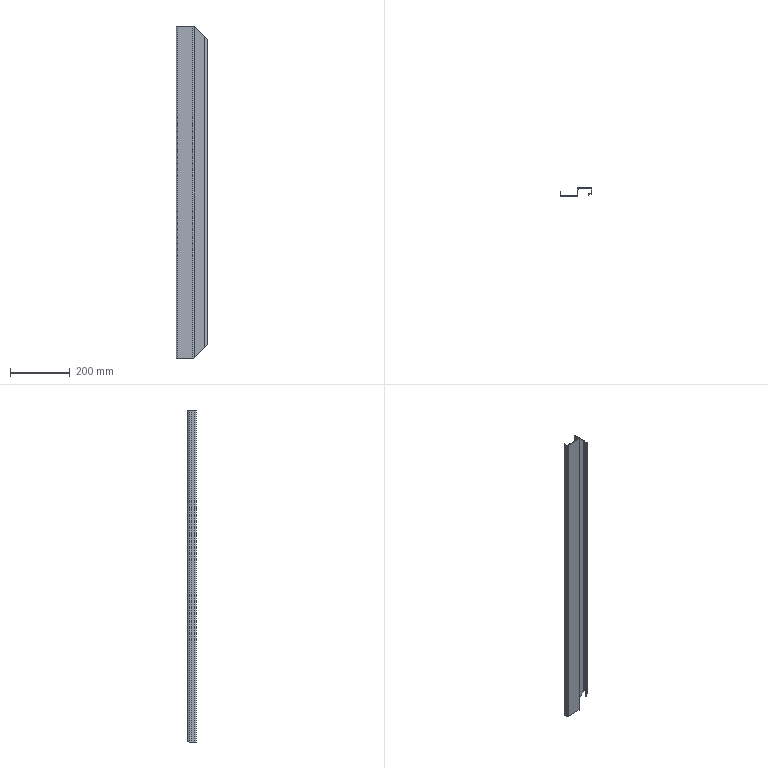Part | STEP file | 750038185 | 1 solid | 38 faces | box 107 x 27 x 1113 mm | volume 364027 mm3 | plane 22 | cylinder 10 | spline 6 | commonest cylinder face diameters 4 x5 8 x5
STEP:
#1=CARTESIAN_POINT('',(-4.,-25.,556.25));
#2=VERTEX_POINT('',#1);
#3=CARTESIAN_POINT('',(-56.,-25.,556.25));
#4=VERTEX_POINT('',#3);
#5=CARTESIAN_POINT('',(0.,-25.,556.25));
#6=DIRECTION('',(-1.,0.,0.));
#7=VECTOR('',#6,1000.);
#8=LINE('',#5,#7);
#9=EDGE_CURVE('',#2,#4,#8,.T.);
#10=ORIENTED_EDGE('',*,*,#9,.T.);
#11=CARTESIAN_POINT('',(-56.,-25.,-556.25));
#12=VERTEX_POINT('',#11);
#13=CARTESIAN_POINT('',(-56.,-25.,556.25));
#14=DIRECTION('',(0.,0.,-1.));
#15=VECTOR('',#14,1000.);
#16=LINE('',#13,#15);
#17=EDGE_CURVE('',#4,#12,#16,.T.);
#18=ORIENTED_EDGE('',*,*,#17,.T.);
#19=CARTESIAN_POINT('',(-4.,-25.,-556.25));
#20=VERTEX_POINT('',#19);
#21=CARTESIAN_POINT('',(0.,-25.,-556.25));
#22=DIRECTION('',(1.,0.,0.));
#23=VECTOR('',#22,1000.);
#24=LINE('',#21,#23);
#25=EDGE_CURVE('',#12,#20,#24,.T.);
#26=ORIENTED_EDGE('',*,*,#25,.T.);
#27=CARTESIAN_POINT('',(-4.,-25.,556.25));
#28=DIRECTION('',(0.,0.,1.));
#29=VECTOR('',#28,1000.);
#30=LINE('',#27,#29);
#31=EDGE_CURVE('',#20,#2,#30,.T.);
#32=ORIENTED_EDGE('',*,*,#31,.T.);
#33=EDGE_LOOP('',(#10,#18,#26,#32));
#34=FACE_OUTER_BOUND('',#33,.T.);
#35=CARTESIAN_POINT('',(0.,-25.,556.25));
#36=DIRECTION('',(0.,-1.,0.));
#37=DIRECTION('',(1.,0.,0.));
#38=AXIS2_PLACEMENT_3D('',#35,#36,#37);
#39=PLANE('',#38);
#40=ADVANCED_FACE('',(#34),#39,.T.);
#41=CARTESIAN_POINT('',(-60.,-21.,556.25));
#42=VERTEX_POINT('',#41);
#43=CARTESIAN_POINT('',(-56.,-21.,556.25));
#44=DIRECTION('',(0.,0.,-1.));
#45=DIRECTION('',(-1.,0.,0.));
#46=AXIS2_PLACEMENT_3D('',#43,#44,#45);
#47=CIRCLE('',#46,4.);
#48=EDGE_CURVE('',#4,#42,#47,.T.);
#49=ORIENTED_EDGE('',*,*,#48,.T.);
#50=CARTESIAN_POINT('',(-60.,-21.,-556.25));
#51=VERTEX_POINT('',#50);
#52=CARTESIAN_POINT('',(-60.,-21.,556.25));
#53=DIRECTION('',(0.,0.,-1.));
#54=VECTOR('',#53,1000.);
#55=LINE('',#52,#54);
#56=EDGE_CURVE('',#42,#51,#55,.T.);
#57=ORIENTED_EDGE('',*,*,#56,.T.);
#58=CARTESIAN_POINT('',(-56.,-21.,-556.25));
#59=DIRECTION('',(0.,0.,1.));
#60=DIRECTION('',(-1.,0.,0.));
#61=AXIS2_PLACEMENT_3D('',#58,#59,#60);
#62=CIRCLE('',#61,4.);
#63=EDGE_CURVE('',#51,#12,#62,.T.);
#64=ORIENTED_EDGE('',*,*,#63,.T.);
#65=ORIENTED_EDGE('',*,*,#17,.F.);
#66=EDGE_LOOP('',(#49,#57,#64,#65));
#67=FACE_OUTER_BOUND('',#66,.T.);
#68=CARTESIAN_POINT('',(-56.,-21.,556.25));
#69=DIRECTION('',(0.,0.,-1.));
#70=DIRECTION('',(-1.,0.,0.));
#71=AXIS2_PLACEMENT_3D('',#68,#69,#70);
#72=CYLINDRICAL_SURFACE('',#71,4.);
#73=ADVANCED_FACE('',(#67),#72,.T.);
#74=CARTESIAN_POINT('',(0.,-21.,556.25));
#75=VERTEX_POINT('',#74);
#76=CARTESIAN_POINT('',(-4.,-21.,556.25));
#77=DIRECTION('',(0.,0.,1.));
#78=DIRECTION('',(-1.,0.,0.));
#79=AXIS2_PLACEMENT_3D('',#76,#77,#78);
#80=CIRCLE('',#79,4.);
#81=EDGE_CURVE('',#2,#75,#80,.T.);
#82=ORIENTED_EDGE('',*,*,#81,.T.);
#83=CARTESIAN_POINT('',(0.,-2.,556.25));
#84=VERTEX_POINT('',#83);
#85=CARTESIAN_POINT('',(0.,-25.,556.25));
#86=DIRECTION('',(0.,1.,0.));
#87=VECTOR('',#86,1000.);
#88=LINE('',#85,#87);
#89=EDGE_CURVE('',#75,#84,#88,.T.);
#90=ORIENTED_EDGE('',*,*,#89,.T.);
#91=CARTESIAN_POINT('',(-2.,-2.,556.25));
#92=VERTEX_POINT('',#91);
#93=CARTESIAN_POINT('',(-60.,-2.,556.25));
#94=DIRECTION('',(-1.,0.,0.));
#95=VECTOR('',#94,1000.);
#96=LINE('',#93,#95);
#97=EDGE_CURVE('',#84,#92,#96,.T.);
#98=ORIENTED_EDGE('',*,*,#97,.T.);
#99=CARTESIAN_POINT('',(-2.,-21.,556.25));
#100=VERTEX_POINT('',#99);
#101=CARTESIAN_POINT('',(-2.,-25.,556.25));
#102=DIRECTION('',(0.,-1.,0.));
#103=VECTOR('',#102,1000.);
#104=LINE('',#101,#103);
#105=EDGE_CURVE('',#92,#100,#104,.T.);
#106=ORIENTED_EDGE('',*,*,#105,.T.);
#107=CARTESIAN_POINT('',(-4.,-23.,556.25));
#108=VERTEX_POINT('',#107);
#109=CARTESIAN_POINT('',(-4.,-21.,556.25));
#110=DIRECTION('',(0.,0.,-1.));
#111=DIRECTION('',(-1.,0.,0.));
#112=AXIS2_PLACEMENT_3D('',#109,#110,#111);
#113=CIRCLE('',#112,2.);
#114=EDGE_CURVE('',#100,#108,#113,.T.);
#115=ORIENTED_EDGE('',*,*,#114,.T.);
#116=CARTESIAN_POINT('',(-56.,-23.,556.25));
#117=VERTEX_POINT('',#116);
#118=CARTESIAN_POINT('',(-60.,-23.,556.25));
#119=DIRECTION('',(-1.,0.,0.));
#120=VECTOR('',#119,1000.);
#121=LINE('',#118,#120);
#122=EDGE_CURVE('',#108,#117,#121,.T.);
#123=ORIENTED_EDGE('',*,*,#122,.T.);
#124=CARTESIAN_POINT('',(-58.,-21.,556.25));
#125=VERTEX_POINT('',#124);
#126=CARTESIAN_POINT('',(-56.,-21.,556.25));
#127=DIRECTION('',(0.,0.,-1.));
#128=DIRECTION('',(-1.,0.,0.));
#129=AXIS2_PLACEMENT_3D('',#126,#127,#128);
#130=CIRCLE('',#129,2.);
#131=EDGE_CURVE('',#117,#125,#130,.T.);
#132=ORIENTED_EDGE('',*,*,#131,.T.);
#133=CARTESIAN_POINT('',(-58.,-10.,556.25));
#134=VERTEX_POINT('',#133);
#135=CARTESIAN_POINT('',(-58.,-25.,556.25));
#136=DIRECTION('',(0.,1.,0.));
#137=VECTOR('',#136,1000.);
#138=LINE('',#135,#137);
#139=EDGE_CURVE('',#125,#134,#138,.T.);
#140=ORIENTED_EDGE('',*,*,#139,.T.);
#141=CARTESIAN_POINT('',(-60.,-10.,556.25));
#142=VERTEX_POINT('',#141);
#143=CARTESIAN_POINT('',(-60.,-10.,556.25));
#144=DIRECTION('',(-1.,0.,0.));
#145=VECTOR('',#144,1000.);
#146=LINE('',#143,#145);
#147=EDGE_CURVE('',#134,#142,#146,.T.);
#148=ORIENTED_EDGE('',*,*,#147,.T.);
#149=CARTESIAN_POINT('',(-60.,-25.,556.25));
#150=DIRECTION('',(0.,-1.,0.));
#151=VECTOR('',#150,1000.);
#152=LINE('',#149,#151);
#153=EDGE_CURVE('',#142,#42,#152,.T.);
#154=ORIENTED_EDGE('',*,*,#153,.T.);
#155=ORIENTED_EDGE('',*,*,#48,.F.);
#156=ORIENTED_EDGE('',*,*,#9,.F.);
#157=EDGE_LOOP('',(#82,#90,#98,#106,#115,#123,#132,#140,#148,#154,#155,#156));
#158=FACE_OUTER_BOUND('',#157,.T.);
#159=CARTESIAN_POINT('',(-60.,-25.,556.25));
#160=DIRECTION('',(0.,0.,1.));
#161=DIRECTION('',(1.,0.,0.));
#162=AXIS2_PLACEMENT_3D('',#159,#160,#161);
#163=PLANE('',#162);
#164=ADVANCED_FACE('',(#158),#163,.T.);
#165=ORIENTED_EDGE('',*,*,#81,.F.);
#166=ORIENTED_EDGE('',*,*,#31,.F.);
#167=CARTESIAN_POINT('',(0.,-21.,-556.25));
#168=VERTEX_POINT('',#167);
#169=CARTESIAN_POINT('',(-4.,-21.,-556.25));
#170=DIRECTION('',(0.,0.,1.));
#171=DIRECTION('',(-1.,0.,0.));
#172=AXIS2_PLACEMENT_3D('',#169,#170,#171);
#173=CIRCLE('',#172,4.);
#174=EDGE_CURVE('',#20,#168,#173,.T.);
#175=ORIENTED_EDGE('',*,*,#174,.T.);
#176=CARTESIAN_POINT('',(0.,-21.,556.25));
#177=DIRECTION('',(0.,0.,1.));
#178=VECTOR('',#177,1000.);
#179=LINE('',#176,#178);
#180=EDGE_CURVE('',#168,#75,#179,.T.);
#181=ORIENTED_EDGE('',*,*,#180,.T.);
#182=EDGE_LOOP('',(#165,#166,#175,#181));
#183=FACE_OUTER_BOUND('',#182,.T.);
#184=CARTESIAN_POINT('',(-4.,-21.,556.25));
#185=DIRECTION('',(0.,0.,-1.));
#186=DIRECTION('',(-1.,0.,0.));
#187=AXIS2_PLACEMENT_3D('',#184,#185,#186);
#188=CYLINDRICAL_SURFACE('',#187,4.);
#189=ADVANCED_FACE('',(#183),#188,.T.);
#190=CARTESIAN_POINT('',(0.,-2.,-556.25));
#191=VERTEX_POINT('',#190);
#192=CARTESIAN_POINT('',(-2.,-2.,-556.25));
#193=VERTEX_POINT('',#192);
#194=CARTESIAN_POINT('',(34.375,-2.,-556.25));
#195=DIRECTION('',(-1.,0.,0.));
#196=VECTOR('',#195,1000.);
#197=LINE('',#194,#196);
#198=EDGE_CURVE('',#191,#193,#197,.T.);
#199=ORIENTED_EDGE('',*,*,#198,.F.);
#200=CARTESIAN_POINT('',(0.,-18.847,-556.25));
#201=DIRECTION('',(0.,1.,0.));
#202=VECTOR('',#201,1000.);
#203=LINE('',#200,#202);
#204=EDGE_CURVE('',#168,#191,#203,.T.);
#205=ORIENTED_EDGE('',*,*,#204,.F.);
#206=ORIENTED_EDGE('',*,*,#174,.F.);
#207=ORIENTED_EDGE('',*,*,#25,.F.);
#208=ORIENTED_EDGE('',*,*,#63,.F.);
#209=CARTESIAN_POINT('',(-60.,-10.,-556.25));
#210=VERTEX_POINT('',#209);
#211=CARTESIAN_POINT('',(-60.,-18.847,-556.25));
#212=DIRECTION('',(0.,-1.,0.));
#213=VECTOR('',#212,1000.);
#214=LINE('',#211,#213);
#215=EDGE_CURVE('',#210,#51,#214,.T.);
#216=ORIENTED_EDGE('',*,*,#215,.F.);
#217=CARTESIAN_POINT('',(-58.,-10.,-556.25));
#218=VERTEX_POINT('',#217);
#219=CARTESIAN_POINT('',(34.375,-10.,-556.25));
#220=DIRECTION('',(-1.,0.,0.));
#221=VECTOR('',#220,1000.);
#222=LINE('',#219,#221);
#223=EDGE_CURVE('',#218,#210,#222,.T.);
#224=ORIENTED_EDGE('',*,*,#223,.F.);
#225=CARTESIAN_POINT('',(-58.,-21.,-556.25));
#226=VERTEX_POINT('',#225);
#227=CARTESIAN_POINT('',(-58.,-18.847,-556.25));
#228=DIRECTION('',(0.,1.,0.));
#229=VECTOR('',#228,1000.);
#230=LINE('',#227,#229);
#231=EDGE_CURVE('',#226,#218,#230,.T.);
#232=ORIENTED_EDGE('',*,*,#231,.F.);
#233=CARTESIAN_POINT('',(-56.,-23.,-556.25));
#234=VERTEX_POINT('',#233);
#235=CARTESIAN_POINT('',(-56.,-21.,-556.25));
#236=DIRECTION('',(0.,0.,-1.));
#237=DIRECTION('',(-1.,0.,0.));
#238=AXIS2_PLACEMENT_3D('',#235,#236,#237);
#239=CIRCLE('',#238,2.);
#240=EDGE_CURVE('',#234,#226,#239,.T.);
#241=ORIENTED_EDGE('',*,*,#240,.F.);
#242=CARTESIAN_POINT('',(-4.,-23.,-556.25));
#243=VERTEX_POINT('',#242);
#244=CARTESIAN_POINT('',(34.375,-23.,-556.25));
#245=DIRECTION('',(-1.,0.,0.));
#246=VECTOR('',#245,1000.);
#247=LINE('',#244,#246);
#248=EDGE_CURVE('',#243,#234,#247,.T.);
#249=ORIENTED_EDGE('',*,*,#248,.F.);
#250=CARTESIAN_POINT('',(-2.,-21.,-556.25));
#251=VERTEX_POINT('',#250);
#252=CARTESIAN_POINT('',(-4.,-21.,-556.25));
#253=DIRECTION('',(0.,0.,-1.));
#254=DIRECTION('',(-1.,0.,0.));
#255=AXIS2_PLACEMENT_3D('',#252,#253,#254);
#256=CIRCLE('',#255,2.);
#257=EDGE_CURVE('',#251,#243,#256,.T.);
#258=ORIENTED_EDGE('',*,*,#257,.F.);
#259=CARTESIAN_POINT('',(-2.,-18.847,-556.25));
#260=DIRECTION('',(0.,-1.,0.));
#261=VECTOR('',#260,1000.);
#262=LINE('',#259,#261);
#263=EDGE_CURVE('',#193,#251,#262,.T.);
#264=ORIENTED_EDGE('',*,*,#263,.F.);
#265=EDGE_LOOP('',(#199,#205,#206,#207,#208,#216,#224,#232,#241,#249,#258,#264));
#266=FACE_OUTER_BOUND('',#265,.T.);
#267=CARTESIAN_POINT('',(34.375,-18.847,-556.25));
#268=DIRECTION('',(0.,0.,1.));
#269=DIRECTION('',(1.,0.,0.));
#270=AXIS2_PLACEMENT_3D('',#267,#268,#269);
#271=PLANE('',#270);
#272=ADVANCED_FACE('',(#266),#271,.F.);
#273=ORIENTED_EDGE('',*,*,#153,.F.);
#274=CARTESIAN_POINT('',(-60.,-10.,556.25));
#275=DIRECTION('',(0.,0.,-1.));
#276=VECTOR('',#275,1000.);
#277=LINE('',#274,#276);
#278=EDGE_CURVE('',#142,#210,#277,.T.);
#279=ORIENTED_EDGE('',*,*,#278,.T.);
#280=ORIENTED_EDGE('',*,*,#215,.T.);
#281=ORIENTED_EDGE('',*,*,#56,.F.);
#282=EDGE_LOOP('',(#273,#279,#280,#281));
#283=FACE_OUTER_BOUND('',#282,.T.);
#284=CARTESIAN_POINT('',(-60.,-25.,556.25));
#285=DIRECTION('',(-1.,0.,0.));
#286=DIRECTION('',(0.,0.,1.));
#287=AXIS2_PLACEMENT_3D('',#284,#285,#286);
#288=PLANE('',#287);
#289=ADVANCED_FACE('',(#283),#288,.T.);
#290=ORIENTED_EDGE('',*,*,#89,.F.);
#291=ORIENTED_EDGE('',*,*,#180,.F.);
#292=ORIENTED_EDGE('',*,*,#204,.T.);
#293=CARTESIAN_POINT('',(0.,-2.,556.25));
#294=DIRECTION('',(0.,0.,1.));
#295=VECTOR('',#294,1000.);
#296=LINE('',#293,#295);
#297=EDGE_CURVE('',#191,#84,#296,.T.);
#298=ORIENTED_EDGE('',*,*,#297,.T.);
#299=EDGE_LOOP('',(#290,#291,#292,#298));
#300=FACE_OUTER_BOUND('',#299,.T.);
#301=CARTESIAN_POINT('',(0.,0.,556.25));
#302=DIRECTION('',(1.,0.,0.));
#303=DIRECTION('',(0.,1.,0.));
#304=AXIS2_PLACEMENT_3D('',#301,#302,#303);
#305=PLANE('',#304);
#306=ADVANCED_FACE('',(#300),#305,.T.);
#307=ORIENTED_EDGE('',*,*,#223,.T.);
#308=ORIENTED_EDGE('',*,*,#278,.F.);
#309=ORIENTED_EDGE('',*,*,#147,.F.);
#310=CARTESIAN_POINT('',(-58.,-10.,556.25));
#311=DIRECTION('',(0.,0.,-1.));
#312=VECTOR('',#311,1000.);
#313=LINE('',#310,#312);
#314=EDGE_CURVE('',#134,#218,#313,.T.);
#315=ORIENTED_EDGE('',*,*,#314,.T.);
#316=EDGE_LOOP('',(#307,#308,#309,#315));
#317=FACE_OUTER_BOUND('',#316,.T.);
#318=CARTESIAN_POINT('',(-60.,-10.,556.25));
#319=DIRECTION('',(0.,1.,0.));
#320=DIRECTION('',(0.,0.,1.));
#321=AXIS2_PLACEMENT_3D('',#318,#319,#320);
#322=PLANE('',#321);
#323=ADVANCED_FACE('',(#317),#322,.T.);
#324=ORIENTED_EDGE('',*,*,#314,.F.);
#325=ORIENTED_EDGE('',*,*,#139,.F.);
#326=CARTESIAN_POINT('',(-58.,-21.,556.25));
#327=DIRECTION('',(0.,0.,1.));
#328=VECTOR('',#327,1000.);
#329=LINE('',#326,#328);
#330=EDGE_CURVE('',#226,#125,#329,.T.);
#331=ORIENTED_EDGE('',*,*,#330,.F.);
#332=ORIENTED_EDGE('',*,*,#231,.T.);
#333=EDGE_LOOP('',(#324,#325,#331,#332));
#334=FACE_OUTER_BOUND('',#333,.T.);
#335=CARTESIAN_POINT('',(-58.,-25.,556.25));
#336=DIRECTION('',(-1.,0.,0.));
#337=DIRECTION('',(0.,0.,1.));
#338=AXIS2_PLACEMENT_3D('',#335,#336,#337);
#339=PLANE('',#338);
#340=ADVANCED_FACE('',(#334),#339,.F.);
#341=ORIENTED_EDGE('',*,*,#330,.T.);
#342=ORIENTED_EDGE('',*,*,#131,.F.);
#343=CARTESIAN_POINT('',(-56.,-23.,556.25));
#344=DIRECTION('',(0.,0.,1.));
#345=VECTOR('',#344,1000.);
#346=LINE('',#343,#345);
#347=EDGE_CURVE('',#234,#117,#346,.T.);
#348=ORIENTED_EDGE('',*,*,#347,.F.);
#349=ORIENTED_EDGE('',*,*,#240,.T.);
#350=EDGE_LOOP('',(#341,#342,#348,#349));
#351=FACE_OUTER_BOUND('',#350,.T.);
#352=CARTESIAN_POINT('',(-56.,-21.,556.25));
#353=DIRECTION('',(0.,0.,-1.));
#354=DIRECTION('',(-1.,0.,0.));
#355=AXIS2_PLACEMENT_3D('',#352,#353,#354);
#356=CYLINDRICAL_SURFACE('',#355,2.);
#357=ADVANCED_FACE('',(#351),#356,.F.);
#358=ORIENTED_EDGE('',*,*,#347,.T.);
#359=ORIENTED_EDGE('',*,*,#122,.F.);
#360=CARTESIAN_POINT('',(-4.,-23.,556.25));
#361=DIRECTION('',(0.,0.,1.));
#362=VECTOR('',#361,1000.);
#363=LINE('',#360,#362);
#364=EDGE_CURVE('',#243,#108,#363,.T.);
#365=ORIENTED_EDGE('',*,*,#364,.F.);
#366=ORIENTED_EDGE('',*,*,#248,.T.);
#367=EDGE_LOOP('',(#358,#359,#365,#366));
#368=FACE_OUTER_BOUND('',#367,.T.);
#369=CARTESIAN_POINT('',(0.,-23.,556.25));
#370=DIRECTION('',(0.,-1.,0.));
#371=DIRECTION('',(1.,0.,0.));
#372=AXIS2_PLACEMENT_3D('',#369,#370,#371);
#373=PLANE('',#372);
#374=ADVANCED_FACE('',(#368),#373,.F.);
#375=ORIENTED_EDGE('',*,*,#364,.T.);
#376=ORIENTED_EDGE('',*,*,#114,.F.);
#377=CARTESIAN_POINT('',(-2.,-21.,556.25));
#378=DIRECTION('',(0.,0.,1.));
#379=VECTOR('',#378,1000.);
#380=LINE('',#377,#379);
#381=EDGE_CURVE('',#251,#100,#380,.T.);
#382=ORIENTED_EDGE('',*,*,#381,.F.);
#383=ORIENTED_EDGE('',*,*,#257,.T.);
#384=EDGE_LOOP('',(#375,#376,#382,#383));
#385=FACE_OUTER_BOUND('',#384,.T.);
#386=CARTESIAN_POINT('',(-4.,-21.,556.25));
#387=DIRECTION('',(0.,0.,-1.));
#388=DIRECTION('',(-1.,0.,0.));
#389=AXIS2_PLACEMENT_3D('',#386,#387,#388);
#390=CYLINDRICAL_SURFACE('',#389,2.);
#391=ADVANCED_FACE('',(#385),#390,.F.);
#392=ORIENTED_EDGE('',*,*,#381,.T.);
#393=ORIENTED_EDGE('',*,*,#105,.F.);
#394=CARTESIAN_POINT('',(-2.,-2.,556.25));
#395=DIRECTION('',(0.,0.,1.));
#396=VECTOR('',#395,1000.);
#397=LINE('',#394,#396);
#398=EDGE_CURVE('',#193,#92,#397,.T.);
#399=ORIENTED_EDGE('',*,*,#398,.F.);
#400=ORIENTED_EDGE('',*,*,#263,.T.);
#401=EDGE_LOOP('',(#392,#393,#399,#400));
#402=FACE_OUTER_BOUND('',#401,.T.);
#403=CARTESIAN_POINT('',(-2.,0.,556.25));
#404=DIRECTION('',(1.,0.,0.));
#405=DIRECTION('',(0.,1.,0.));
#406=AXIS2_PLACEMENT_3D('',#403,#404,#405);
#407=PLANE('',#406);
#408=ADVANCED_FACE('',(#402),#407,.F.);
#409=CARTESIAN_POINT('',(2.,0.,554.25));
#410=VERTEX_POINT('',#409);
#411=CARTESIAN_POINT('',(2.,2.,554.25));
#412=VERTEX_POINT('',#411);
#413=CARTESIAN_POINT('',(2.,1.,554.25));
#414=DIRECTION('',(0.,1.,0.));
#415=VECTOR('',#414,1000.);
#416=LINE('',#413,#415);
#417=EDGE_CURVE('',#410,#412,#416,.T.);
#418=ORIENTED_EDGE('',*,*,#417,.T.);
#419=CARTESIAN_POINT('',(2.,2.,554.25));
#420=CARTESIAN_POINT('',(-0.6667,2.,555.583));
#421=CARTESIAN_POINT('',(-2.,0.,556.25));
#422=CARTESIAN_POINT('',(-2.,-2.,556.25));
#423=(BOUNDED_CURVE()B_SPLINE_CURVE(3,(#419,#420,#421,#422),.UNSPECIFIED.,.F.,.F.)B_SPLINE_CURVE_WITH_KNOTS((4,4),(0.,0.006622),.UNSPECIFIED.)CURVE()GEOMETRIC_REPRESENTATION_ITEM()RATIONAL_B_SPLINE_CURVE((0.5,0.5,0.6667,1.))REPRESENTATION_ITEM(''));
#424=EDGE_CURVE('',#412,#92,#423,.T.);
#425=ORIENTED_EDGE('',*,*,#424,.T.);
#426=ORIENTED_EDGE('',*,*,#97,.F.);
#427=CARTESIAN_POINT('',(0.,-2.,556.25));
#428=CARTESIAN_POINT('',(0.,-1.,556.25));
#429=CARTESIAN_POINT('',(0.6667,0.,555.583));
#430=CARTESIAN_POINT('',(2.,0.,554.25));
#431=(BOUNDED_CURVE()B_SPLINE_CURVE(3,(#427,#428,#429,#430),.UNSPECIFIED.,.F.,.F.)B_SPLINE_CURVE_WITH_KNOTS((4,4),(0.,0.003854),.UNSPECIFIED.)CURVE()GEOMETRIC_REPRESENTATION_ITEM()RATIONAL_B_SPLINE_CURVE((1.,0.6667,0.5,0.5))REPRESENTATION_ITEM(''));
#432=EDGE_CURVE('',#84,#410,#431,.T.);
#433=ORIENTED_EDGE('',*,*,#432,.T.);
#434=EDGE_LOOP('',(#418,#425,#426,#433));
#435=FACE_OUTER_BOUND('',#434,.T.);
#436=CARTESIAN_POINT('',(4.,-2.,552.25));
#437=CARTESIAN_POINT('',(4.667,-2.,552.25));
#438=CARTESIAN_POINT('',(5.333,-2.,552.25));
#439=CARTESIAN_POINT('',(6.,-2.,552.25));
#440=CARTESIAN_POINT('',(4.,-6.,552.25));
#441=CARTESIAN_POINT('',(4.667,-7.333,552.25));
#442=CARTESIAN_POINT('',(5.333,-8.667,552.25));
#443=CARTESIAN_POINT('',(6.,-10.,552.25));
#444=CARTESIAN_POINT('',(0.,-6.,556.25));
#445=CARTESIAN_POINT('',(-0.6667,-7.333,556.25));
#446=CARTESIAN_POINT('',(-1.333,-8.667,556.25));
#447=CARTESIAN_POINT('',(-2.,-10.,556.25));
#448=CARTESIAN_POINT('',(0.,-2.,556.25));
#449=CARTESIAN_POINT('',(-0.6667,-2.,556.25));
#450=CARTESIAN_POINT('',(-1.333,-2.,556.25));
#451=CARTESIAN_POINT('',(-2.,-2.,556.25));
#452=CARTESIAN_POINT('',(0.,2.,556.25));
#453=CARTESIAN_POINT('',(-0.6667,3.333,556.25));
#454=CARTESIAN_POINT('',(-1.333,4.667,556.25));
#455=CARTESIAN_POINT('',(-2.,6.,556.25));
#456=CARTESIAN_POINT('',(4.,2.,552.25));
#457=CARTESIAN_POINT('',(4.667,3.333,552.25));
#458=CARTESIAN_POINT('',(5.333,4.667,552.25));
#459=CARTESIAN_POINT('',(6.,6.,552.25));
#460=CARTESIAN_POINT('',(4.,-2.,552.25));
#461=CARTESIAN_POINT('',(4.667,-2.,552.25));
#462=CARTESIAN_POINT('',(5.333,-2.,552.25));
#463=CARTESIAN_POINT('',(6.,-2.,552.25));
#464=(BOUNDED_SURFACE()B_SPLINE_SURFACE(3,3,((#436,#437,#438,#439),(#440,#441,#442,#443),(#444,#445,#446,#447),(#448,#449,#450,#451),(#452,#453,#454,#455),(#456,#457,#458,#459),(#460,#461,#462,#463)),.UNSPECIFIED.,.T.,.F.,.F.)B_SPLINE_SURFACE_WITH_KNOTS((4,3,4),(4,4),(0.,0.5,1.),(0.,1.),.UNSPECIFIED.)GEOMETRIC_REPRESENTATION_ITEM()RATIONAL_B_SPLINE_SURFACE(((1.,1.,1.,1.),(0.3333,0.3333,0.3333,0.3333),(0.3333,0.3333,0.3333,0.3333),(1.,1.,1.,1.),(0.3333,0.3333,0.3333,0.3333),(0.3333,0.3333,0.3333,0.3333),(1.,1.,1.,1.)))REPRESENTATION_ITEM('')SURFACE());
#465=ADVANCED_FACE('',(#435),#464,.T.);
#466=ORIENTED_EDGE('',*,*,#198,.T.);
#467=CARTESIAN_POINT('',(2.,2.,-554.25));
#468=VERTEX_POINT('',#467);
#469=CARTESIAN_POINT('',(-2.,-2.,-556.25));
#470=CARTESIAN_POINT('',(-2.,0.,-556.25));
#471=CARTESIAN_POINT('',(-0.6667,2.,-555.583));
#472=CARTESIAN_POINT('',(2.,2.,-554.25));
#473=(BOUNDED_CURVE()B_SPLINE_CURVE(3,(#469,#470,#471,#472),.UNSPECIFIED.,.F.,.F.)B_SPLINE_CURVE_WITH_KNOTS((4,4),(0.,0.006696),.UNSPECIFIED.)CURVE()GEOMETRIC_REPRESENTATION_ITEM()RATIONAL_B_SPLINE_CURVE((1.,0.6667,0.5,0.5))REPRESENTATION_ITEM(''));
#474=EDGE_CURVE('',#193,#468,#473,.T.);
#475=ORIENTED_EDGE('',*,*,#474,.T.);
#476=CARTESIAN_POINT('',(2.,0.,-554.25));
#477=VERTEX_POINT('',#476);
#478=CARTESIAN_POINT('',(2.,1.,-554.25));
#479=DIRECTION('',(0.,-1.,0.));
#480=VECTOR('',#479,1000.);
#481=LINE('',#478,#480);
#482=EDGE_CURVE('',#468,#477,#481,.T.);
#483=ORIENTED_EDGE('',*,*,#482,.T.);
#484=CARTESIAN_POINT('',(2.,0.,-554.25));
#485=CARTESIAN_POINT('',(0.6667,0.,-555.583));
#486=CARTESIAN_POINT('',(0.,-1.,-556.25));
#487=CARTESIAN_POINT('',(0.,-2.,-556.25));
#488=(BOUNDED_CURVE()B_SPLINE_CURVE(3,(#484,#485,#486,#487),.UNSPECIFIED.,.F.,.T.)B_SPLINE_CURVE_WITH_KNOTS((4,4),(0.,0.003785),.UNSPECIFIED.)CURVE()GEOMETRIC_REPRESENTATION_ITEM()RATIONAL_B_SPLINE_CURVE((0.5,0.5,0.6667,1.))REPRESENTATION_ITEM(''));
#489=EDGE_CURVE('',#477,#191,#488,.T.);
#490=ORIENTED_EDGE('',*,*,#489,.T.);
#491=EDGE_LOOP('',(#466,#475,#483,#490));
#492=FACE_OUTER_BOUND('',#491,.T.);
#493=CARTESIAN_POINT('',(0.,-2.,-556.25));
#494=CARTESIAN_POINT('',(-0.6667,-2.,-556.25));
#495=CARTESIAN_POINT('',(-1.333,-2.,-556.25));
#496=CARTESIAN_POINT('',(-2.,-2.,-556.25));
#497=CARTESIAN_POINT('',(0.,-6.,-556.25));
#498=CARTESIAN_POINT('',(-0.6667,-7.333,-556.25));
#499=CARTESIAN_POINT('',(-1.333,-8.667,-556.25));
#500=CARTESIAN_POINT('',(-2.,-10.,-556.25));
#501=CARTESIAN_POINT('',(4.,-6.,-552.25));
#502=CARTESIAN_POINT('',(4.667,-7.333,-552.25));
#503=CARTESIAN_POINT('',(5.333,-8.667,-552.25));
#504=CARTESIAN_POINT('',(6.,-10.,-552.25));
#505=CARTESIAN_POINT('',(4.,-2.,-552.25));
#506=CARTESIAN_POINT('',(4.667,-2.,-552.25));
#507=CARTESIAN_POINT('',(5.333,-2.,-552.25));
#508=CARTESIAN_POINT('',(6.,-2.,-552.25));
#509=CARTESIAN_POINT('',(4.,2.,-552.25));
#510=CARTESIAN_POINT('',(4.667,3.333,-552.25));
#511=CARTESIAN_POINT('',(5.333,4.667,-552.25));
#512=CARTESIAN_POINT('',(6.,6.,-552.25));
#513=CARTESIAN_POINT('',(0.,2.,-556.25));
#514=CARTESIAN_POINT('',(-0.6667,3.333,-556.25));
#515=CARTESIAN_POINT('',(-1.333,4.667,-556.25));
#516=CARTESIAN_POINT('',(-2.,6.,-556.25));
#517=CARTESIAN_POINT('',(0.,-2.,-556.25));
#518=CARTESIAN_POINT('',(-0.6667,-2.,-556.25));
#519=CARTESIAN_POINT('',(-1.333,-2.,-556.25));
#520=CARTESIAN_POINT('',(-2.,-2.,-556.25));
#521=(BOUNDED_SURFACE()B_SPLINE_SURFACE(3,3,((#493,#494,#495,#496),(#497,#498,#499,#500),(#501,#502,#503,#504),(#505,#506,#507,#508),(#509,#510,#511,#512),(#513,#514,#515,#516),(#517,#518,#519,#520)),.UNSPECIFIED.,.T.,.F.,.F.)B_SPLINE_SURFACE_WITH_KNOTS((4,3,4),(4,4),(0.,0.5,1.),(0.,1.),.UNSPECIFIED.)GEOMETRIC_REPRESENTATION_ITEM()RATIONAL_B_SPLINE_SURFACE(((1.,1.,1.,1.),(0.3333,0.3333,0.3333,0.3333),(0.3333,0.3333,0.3333,0.3333),(1.,1.,1.,1.),(0.3333,0.3333,0.3333,0.3333),(0.3333,0.3333,0.3333,0.3333),(1.,1.,1.,1.)))REPRESENTATION_ITEM('')SURFACE());
#522=ADVANCED_FACE('',(#492),#521,.T.);
#523=ORIENTED_EDGE('',*,*,#297,.F.);
#524=ORIENTED_EDGE('',*,*,#489,.F.);
#525=CARTESIAN_POINT('',(2.,0.,556.25));
#526=DIRECTION('',(0.,0.,-1.));
#527=VECTOR('',#526,1000.);
#528=LINE('',#525,#527);
#529=EDGE_CURVE('',#410,#477,#528,.T.);
#530=ORIENTED_EDGE('',*,*,#529,.F.);
#531=ORIENTED_EDGE('',*,*,#432,.F.);
#532=EDGE_LOOP('',(#523,#524,#530,#531));
#533=FACE_OUTER_BOUND('',#532,.T.);
#534=CARTESIAN_POINT('',(2.,-2.,556.25));
#535=DIRECTION('',(0.,0.,-1.));
#536=DIRECTION('',(-1.,0.,0.));
#537=AXIS2_PLACEMENT_3D('',#534,#535,#536);
#538=CYLINDRICAL_SURFACE('',#537,2.);
#539=ADVANCED_FACE('',(#533),#538,.F.);
#540=CARTESIAN_POINT('',(2.,2.,556.25));
#541=DIRECTION('',(0.,0.,-1.));
#542=VECTOR('',#541,1000.);
#543=LINE('',#540,#542);
#544=EDGE_CURVE('',#412,#468,#543,.T.);
#545=ORIENTED_EDGE('',*,*,#544,.T.);
#546=ORIENTED_EDGE('',*,*,#474,.F.);
#547=ORIENTED_EDGE('',*,*,#398,.T.);
#548=ORIENTED_EDGE('',*,*,#424,.F.);
#549=EDGE_LOOP('',(#545,#546,#547,#548));
#550=FACE_OUTER_BOUND('',#549,.T.);
#551=CARTESIAN_POINT('',(2.,-2.,556.25));
#552=DIRECTION('',(0.,0.,-1.));
#553=DIRECTION('',(-1.,0.,0.));
#554=AXIS2_PLACEMENT_3D('',#551,#552,#553);
#555=CYLINDRICAL_SURFACE('',#554,4.);
#556=ADVANCED_FACE('',(#550),#555,.T.);
#557=CARTESIAN_POINT('',(43.,0.,513.25));
#558=VERTEX_POINT('',#557);
#559=CARTESIAN_POINT('',(22.5,0.,533.75));
#560=DIRECTION('',(-0.7071,0.,0.7071));
#561=VECTOR('',#560,1000.);
#562=LINE('',#559,#561);
#563=EDGE_CURVE('',#558,#410,#562,.T.);
#564=ORIENTED_EDGE('',*,*,#563,.F.);
#565=CARTESIAN_POINT('',(43.,2.,513.25));
#566=VERTEX_POINT('',#565);
#567=CARTESIAN_POINT('',(43.,0.,513.25));
#568=DIRECTION('',(0.,-1.,0.));
#569=VECTOR('',#568,1000.);
#570=LINE('',#567,#569);
#571=EDGE_CURVE('',#566,#558,#570,.T.);
#572=ORIENTED_EDGE('',*,*,#571,.F.);
#573=CARTESIAN_POINT('',(22.5,2.,533.75));
#574=DIRECTION('',(0.7071,0.,-0.7071));
#575=VECTOR('',#574,1000.);
#576=LINE('',#573,#575);
#577=EDGE_CURVE('',#412,#566,#576,.T.);
#578=ORIENTED_EDGE('',*,*,#577,.F.);
#579=ORIENTED_EDGE('',*,*,#417,.F.);
#580=EDGE_LOOP('',(#564,#572,#578,#579));
#581=FACE_OUTER_BOUND('',#580,.T.);
#582=CARTESIAN_POINT('',(22.5,0.,533.75));
#583=DIRECTION('',(-0.7071,0.,-0.7071));
#584=DIRECTION('',(-0.7071,0.,0.7071));
#585=AXIS2_PLACEMENT_3D('',#582,#583,#584);
#586=PLANE('',#585);
#587=ADVANCED_FACE('',(#581),#586,.F.);
#588=CARTESIAN_POINT('',(43.,0.,-513.25));
#589=VERTEX_POINT('',#588);
#590=CARTESIAN_POINT('',(578.75,0.,22.5));
#591=DIRECTION('',(0.7071,0.,0.7071));
#592=VECTOR('',#591,1000.);
#593=LINE('',#590,#592);
#594=EDGE_CURVE('',#477,#589,#593,.T.);
#595=ORIENTED_EDGE('',*,*,#594,.F.);
#596=ORIENTED_EDGE('',*,*,#482,.F.);
#597=CARTESIAN_POINT('',(43.,2.,-513.25));
#598=VERTEX_POINT('',#597);
#599=CARTESIAN_POINT('',(578.75,2.,22.5));
#600=DIRECTION('',(-0.7071,0.,-0.7071));
#601=VECTOR('',#600,1000.);
#602=LINE('',#599,#601);
#603=EDGE_CURVE('',#598,#468,#602,.T.);
#604=ORIENTED_EDGE('',*,*,#603,.F.);
#605=CARTESIAN_POINT('',(43.,0.,-513.25));
#606=DIRECTION('',(0.,1.,0.));
#607=VECTOR('',#606,1000.);
#608=LINE('',#605,#607);
#609=EDGE_CURVE('',#589,#598,#608,.T.);
#610=ORIENTED_EDGE('',*,*,#609,.F.);
#611=EDGE_LOOP('',(#595,#596,#604,#610));
#612=FACE_OUTER_BOUND('',#611,.T.);
#613=CARTESIAN_POINT('',(578.75,0.,22.5));
#614=DIRECTION('',(-0.7071,0.,0.7071));
#615=DIRECTION('',(0.7071,0.,0.7071));
#616=AXIS2_PLACEMENT_3D('',#613,#614,#615);
#617=PLANE('',#616);
#618=ADVANCED_FACE('',(#612),#617,.F.);
#619=ORIENTED_EDGE('',*,*,#594,.T.);
#620=CARTESIAN_POINT('',(43.,0.,556.25));
#621=DIRECTION('',(0.,0.,1.));
#622=VECTOR('',#621,1000.);
#623=LINE('',#620,#622);
#624=EDGE_CURVE('',#589,#558,#623,.T.);
#625=ORIENTED_EDGE('',*,*,#624,.T.);
#626=ORIENTED_EDGE('',*,*,#563,.T.);
#627=ORIENTED_EDGE('',*,*,#529,.T.);
#628=EDGE_LOOP('',(#619,#625,#626,#627));
#629=FACE_OUTER_BOUND('',#628,.T.);
#630=CARTESIAN_POINT('',(45.,0.,556.25));
#631=DIRECTION('',(0.,-1.,0.));
#632=DIRECTION('',(0.,0.,-1.));
#633=AXIS2_PLACEMENT_3D('',#630,#631,#632);
#634=PLANE('',#633);
#635=ADVANCED_FACE('',(#629),#634,.T.);
#636=ORIENTED_EDGE('',*,*,#577,.T.);
#637=CARTESIAN_POINT('',(43.,2.,556.25));
#638=DIRECTION('',(0.,0.,1.));
#639=VECTOR('',#638,1000.);
#640=LINE('',#637,#639);
#641=EDGE_CURVE('',#598,#566,#640,.T.);
#642=ORIENTED_EDGE('',*,*,#641,.F.);
#643=ORIENTED_EDGE('',*,*,#603,.T.);
#644=ORIENTED_EDGE('',*,*,#544,.F.);
#645=EDGE_LOOP('',(#636,#642,#643,#644));
#646=FACE_OUTER_BOUND('',#645,.T.);
#647=CARTESIAN_POINT('',(45.,2.,556.25));
#648=DIRECTION('',(0.,-1.,0.));
#649=DIRECTION('',(0.,0.,-1.));
#650=AXIS2_PLACEMENT_3D('',#647,#648,#649);
#651=PLANE('',#650);
#652=ADVANCED_FACE('',(#646),#651,.F.);
#653=CARTESIAN_POINT('',(47.,-2.,509.25));
#654=VERTEX_POINT('',#653);
#655=CARTESIAN_POINT('',(47.,-2.,509.25));
#656=CARTESIAN_POINT('',(47.,0.,509.25));
#657=CARTESIAN_POINT('',(45.667,2.,510.583));
#658=CARTESIAN_POINT('',(43.,2.,513.25));
#659=(BOUNDED_CURVE()B_SPLINE_CURVE(3,(#655,#656,#657,#658),.UNSPECIFIED.,.F.,.F.)B_SPLINE_CURVE_WITH_KNOTS((4,4),(0.,0.007712),.UNSPECIFIED.)CURVE()GEOMETRIC_REPRESENTATION_ITEM()RATIONAL_B_SPLINE_CURVE((1.,0.6667,0.5,0.5))REPRESENTATION_ITEM(''));
#660=EDGE_CURVE('',#654,#566,#659,.T.);
#661=ORIENTED_EDGE('',*,*,#660,.T.);
#662=ORIENTED_EDGE('',*,*,#571,.T.);
#663=CARTESIAN_POINT('',(45.,-2.,509.25));
#664=VERTEX_POINT('',#663);
#665=CARTESIAN_POINT('',(43.,0.,513.25));
#666=CARTESIAN_POINT('',(44.333,0.,510.583));
#667=CARTESIAN_POINT('',(45.,-1.,509.25));
#668=CARTESIAN_POINT('',(45.,-2.,509.25));
#669=(BOUNDED_CURVE()B_SPLINE_CURVE(3,(#665,#666,#667,#668),.UNSPECIFIED.,.F.,.F.)B_SPLINE_CURVE_WITH_KNOTS((4,4),(0.,0.005228),.UNSPECIFIED.)CURVE()GEOMETRIC_REPRESENTATION_ITEM()RATIONAL_B_SPLINE_CURVE((0.5,0.5,0.6667,1.))REPRESENTATION_ITEM(''));
#670=EDGE_CURVE('',#558,#664,#669,.T.);
#671=ORIENTED_EDGE('',*,*,#670,.T.);
#672=CARTESIAN_POINT('',(46.,-2.,509.25));
#673=DIRECTION('',(1.,0.,0.));
#674=VECTOR('',#673,1000.);
#675=LINE('',#672,#674);
#676=EDGE_CURVE('',#664,#654,#675,.T.);
#677=ORIENTED_EDGE('',*,*,#676,.T.);
#678=EDGE_LOOP('',(#661,#662,#671,#677));
#679=FACE_OUTER_BOUND('',#678,.T.);
#680=CARTESIAN_POINT('',(45.,-2.,509.25));
#681=CARTESIAN_POINT('',(45.667,-2.,509.25));
#682=CARTESIAN_POINT('',(46.333,-2.,509.25));
#683=CARTESIAN_POINT('',(47.,-2.,509.25));
#684=CARTESIAN_POINT('',(45.,-6.,509.25));
#685=CARTESIAN_POINT('',(45.667,-7.333,509.25));
#686=CARTESIAN_POINT('',(46.333,-8.667,509.25));
#687=CARTESIAN_POINT('',(47.,-10.,509.25));
#688=CARTESIAN_POINT('',(41.,-6.,517.25));
#689=CARTESIAN_POINT('',(40.333,-7.333,517.25));
#690=CARTESIAN_POINT('',(39.667,-8.667,517.25));
#691=CARTESIAN_POINT('',(39.,-10.,517.25));
#692=CARTESIAN_POINT('',(41.,-2.,517.25));
#693=CARTESIAN_POINT('',(40.333,-2.,517.25));
#694=CARTESIAN_POINT('',(39.667,-2.,517.25));
#695=CARTESIAN_POINT('',(39.,-2.,517.25));
#696=CARTESIAN_POINT('',(41.,2.,517.25));
#697=CARTESIAN_POINT('',(40.333,3.333,517.25));
#698=CARTESIAN_POINT('',(39.667,4.667,517.25));
#699=CARTESIAN_POINT('',(39.,6.,517.25));
#700=CARTESIAN_POINT('',(45.,2.,509.25));
#701=CARTESIAN_POINT('',(45.667,3.333,509.25));
#702=CARTESIAN_POINT('',(46.333,4.667,509.25));
#703=CARTESIAN_POINT('',(47.,6.,509.25));
#704=CARTESIAN_POINT('',(45.,-2.,509.25));
#705=CARTESIAN_POINT('',(45.667,-2.,509.25));
#706=CARTESIAN_POINT('',(46.333,-2.,509.25));
#707=CARTESIAN_POINT('',(47.,-2.,509.25));
#708=(BOUNDED_SURFACE()B_SPLINE_SURFACE(3,3,((#680,#681,#682,#683),(#684,#685,#686,#687),(#688,#689,#690,#691),(#692,#693,#694,#695),(#696,#697,#698,#699),(#700,#701,#702,#703),(#704,#705,#706,#707)),.UNSPECIFIED.,.T.,.F.,.T.)B_SPLINE_SURFACE_WITH_KNOTS((4,3,4),(4,4),(0.,0.5,1.),(0.,1.),.UNSPECIFIED.)GEOMETRIC_REPRESENTATION_ITEM()RATIONAL_B_SPLINE_SURFACE(((1.,1.,1.,1.),(0.3333,0.3333,0.3333,0.3333),(0.3333,0.3333,0.3333,0.3333),(1.,1.,1.,1.),(0.3333,0.3333,0.3333,0.3333),(0.3333,0.3333,0.3333,0.3333),(1.,1.,1.,1.)))REPRESENTATION_ITEM('')SURFACE());
#709=ADVANCED_FACE('',(#679),#708,.T.);
#710=CARTESIAN_POINT('',(47.,-2.,-509.25));
#711=VERTEX_POINT('',#710);
#712=CARTESIAN_POINT('',(45.,-2.,-509.25));
#713=VERTEX_POINT('',#712);
#714=CARTESIAN_POINT('',(46.,-2.,-509.25));
#715=DIRECTION('',(-1.,0.,0.));
#716=VECTOR('',#715,1000.);
#717=LINE('',#714,#716);
#718=EDGE_CURVE('',#711,#713,#717,.T.);
#719=ORIENTED_EDGE('',*,*,#718,.T.);
#720=CARTESIAN_POINT('',(45.,-2.,-509.25));
#721=CARTESIAN_POINT('',(45.,-1.,-509.25));
#722=CARTESIAN_POINT('',(44.333,0.,-510.583));
#723=CARTESIAN_POINT('',(43.,0.,-513.25));
#724=(BOUNDED_CURVE()B_SPLINE_CURVE(3,(#720,#721,#722,#723),.UNSPECIFIED.,.F.,.T.)B_SPLINE_CURVE_WITH_KNOTS((4,4),(0.,0.00529),.UNSPECIFIED.)CURVE()GEOMETRIC_REPRESENTATION_ITEM()RATIONAL_B_SPLINE_CURVE((1.,0.6667,0.5,0.5))REPRESENTATION_ITEM(''));
#725=EDGE_CURVE('',#713,#589,#724,.T.);
#726=ORIENTED_EDGE('',*,*,#725,.T.);
#727=ORIENTED_EDGE('',*,*,#609,.T.);
#728=CARTESIAN_POINT('',(43.,2.,-513.25));
#729=CARTESIAN_POINT('',(45.667,2.,-510.583));
#730=CARTESIAN_POINT('',(47.,0.,-509.25));
#731=CARTESIAN_POINT('',(47.,-2.,-509.25));
#732=(BOUNDED_CURVE()B_SPLINE_CURVE(3,(#728,#729,#730,#731),.UNSPECIFIED.,.F.,.F.)B_SPLINE_CURVE_WITH_KNOTS((4,4),(0.,0.007567),.UNSPECIFIED.)CURVE()GEOMETRIC_REPRESENTATION_ITEM()RATIONAL_B_SPLINE_CURVE((0.5,0.5,0.6667,1.))REPRESENTATION_ITEM(''));
#733=EDGE_CURVE('',#598,#711,#732,.T.);
#734=ORIENTED_EDGE('',*,*,#733,.T.);
#735=EDGE_LOOP('',(#719,#726,#727,#734));
#736=FACE_OUTER_BOUND('',#735,.T.);
#737=CARTESIAN_POINT('',(41.,-2.,-517.25));
#738=CARTESIAN_POINT('',(40.333,-2.,-517.25));
#739=CARTESIAN_POINT('',(39.667,-2.,-517.25));
#740=CARTESIAN_POINT('',(39.,-2.,-517.25));
#741=CARTESIAN_POINT('',(41.,-6.,-517.25));
#742=CARTESIAN_POINT('',(40.333,-7.333,-517.25));
#743=CARTESIAN_POINT('',(39.667,-8.667,-517.25));
#744=CARTESIAN_POINT('',(39.,-10.,-517.25));
#745=CARTESIAN_POINT('',(45.,-6.,-509.25));
#746=CARTESIAN_POINT('',(45.667,-7.333,-509.25));
#747=CARTESIAN_POINT('',(46.333,-8.667,-509.25));
#748=CARTESIAN_POINT('',(47.,-10.,-509.25));
#749=CARTESIAN_POINT('',(45.,-2.,-509.25));
#750=CARTESIAN_POINT('',(45.667,-2.,-509.25));
#751=CARTESIAN_POINT('',(46.333,-2.,-509.25));
#752=CARTESIAN_POINT('',(47.,-2.,-509.25));
#753=CARTESIAN_POINT('',(45.,2.,-509.25));
#754=CARTESIAN_POINT('',(45.667,3.333,-509.25));
#755=CARTESIAN_POINT('',(46.333,4.667,-509.25));
#756=CARTESIAN_POINT('',(47.,6.,-509.25));
#757=CARTESIAN_POINT('',(41.,2.,-517.25));
#758=CARTESIAN_POINT('',(40.333,3.333,-517.25));
#759=CARTESIAN_POINT('',(39.667,4.667,-517.25));
#760=CARTESIAN_POINT('',(39.,6.,-517.25));
#761=CARTESIAN_POINT('',(41.,-2.,-517.25));
#762=CARTESIAN_POINT('',(40.333,-2.,-517.25));
#763=CARTESIAN_POINT('',(39.667,-2.,-517.25));
#764=CARTESIAN_POINT('',(39.,-2.,-517.25));
#765=(BOUNDED_SURFACE()B_SPLINE_SURFACE(3,3,((#737,#738,#739,#740),(#741,#742,#743,#744),(#745,#746,#747,#748),(#749,#750,#751,#752),(#753,#754,#755,#756),(#757,#758,#759,#760),(#761,#762,#763,#764)),.UNSPECIFIED.,.T.,.F.,.F.)B_SPLINE_SURFACE_WITH_KNOTS((4,3,4),(4,4),(0.,0.5,1.),(0.,1.),.UNSPECIFIED.)GEOMETRIC_REPRESENTATION_ITEM()RATIONAL_B_SPLINE_SURFACE(((1.,1.,1.,1.),(0.3333,0.3333,0.3333,0.3333),(0.3333,0.3333,0.3333,0.3333),(1.,1.,1.,1.),(0.3333,0.3333,0.3333,0.3333),(0.3333,0.3333,0.3333,0.3333),(1.,1.,1.,1.)))REPRESENTATION_ITEM('')SURFACE());
#766=ADVANCED_FACE('',(#736),#765,.T.);
#767=ORIENTED_EDGE('',*,*,#624,.F.);
#768=ORIENTED_EDGE('',*,*,#725,.F.);
#769=CARTESIAN_POINT('',(45.,-2.,556.25));
#770=DIRECTION('',(0.,0.,-1.));
#771=VECTOR('',#770,1000.);
#772=LINE('',#769,#771);
#773=EDGE_CURVE('',#664,#713,#772,.T.);
#774=ORIENTED_EDGE('',*,*,#773,.F.);
#775=ORIENTED_EDGE('',*,*,#670,.F.);
#776=EDGE_LOOP('',(#767,#768,#774,#775));
#777=FACE_OUTER_BOUND('',#776,.T.);
#778=CARTESIAN_POINT('',(43.,-2.,556.25));
#779=DIRECTION('',(0.,0.,-1.));
#780=DIRECTION('',(-1.,0.,0.));
#781=AXIS2_PLACEMENT_3D('',#778,#779,#780);
#782=CYLINDRICAL_SURFACE('',#781,2.);
#783=ADVANCED_FACE('',(#777),#782,.F.);
#784=CARTESIAN_POINT('',(47.,-2.,556.25));
#785=DIRECTION('',(0.,0.,-1.));
#786=VECTOR('',#785,1000.);
#787=LINE('',#784,#786);
#788=EDGE_CURVE('',#654,#711,#787,.T.);
#789=ORIENTED_EDGE('',*,*,#788,.T.);
#790=ORIENTED_EDGE('',*,*,#733,.F.);
#791=ORIENTED_EDGE('',*,*,#641,.T.);
#792=ORIENTED_EDGE('',*,*,#660,.F.);
#793=EDGE_LOOP('',(#789,#790,#791,#792));
#794=FACE_OUTER_BOUND('',#793,.T.);
#795=CARTESIAN_POINT('',(43.,-2.,556.25));
#796=DIRECTION('',(0.,0.,-1.));
#797=DIRECTION('',(-1.,0.,0.));
#798=AXIS2_PLACEMENT_3D('',#795,#796,#797);
#799=CYLINDRICAL_SURFACE('',#798,4.);
#800=ADVANCED_FACE('',(#794),#799,.T.);
#801=CARTESIAN_POINT('',(47.,-14.465,509.25));
#802=VERTEX_POINT('',#801);
#803=CARTESIAN_POINT('',(47.,-16.,509.25));
#804=DIRECTION('',(0.,-1.,0.));
#805=VECTOR('',#804,1000.);
#806=LINE('',#803,#805);
#807=EDGE_CURVE('',#654,#802,#806,.T.);
#808=ORIENTED_EDGE('',*,*,#807,.F.);
#809=ORIENTED_EDGE('',*,*,#676,.F.);
#810=CARTESIAN_POINT('',(45.,-14.465,509.25));
#811=VERTEX_POINT('',#810);
#812=CARTESIAN_POINT('',(45.,-16.,509.25));
#813=DIRECTION('',(0.,1.,0.));
#814=VECTOR('',#813,1000.);
#815=LINE('',#812,#814);
#816=EDGE_CURVE('',#811,#664,#815,.T.);
#817=ORIENTED_EDGE('',*,*,#816,.F.);
#818=CARTESIAN_POINT('',(47.,-14.465,509.25));
#819=DIRECTION('',(-1.,0.,0.));
#820=VECTOR('',#819,1000.);
#821=LINE('',#818,#820);
#822=EDGE_CURVE('',#802,#811,#821,.T.);
#823=ORIENTED_EDGE('',*,*,#822,.F.);
#824=EDGE_LOOP('',(#808,#809,#817,#823));
#825=FACE_OUTER_BOUND('',#824,.T.);
#826=CARTESIAN_POINT('',(47.,-16.,509.25));
#827=DIRECTION('',(0.,0.,-1.));
#828=DIRECTION('',(0.,1.,0.));
#829=AXIS2_PLACEMENT_3D('',#826,#827,#828);
#830=PLANE('',#829);
#831=ADVANCED_FACE('',(#825),#830,.F.);
#832=CARTESIAN_POINT('',(47.,-14.465,-509.25));
#833=VERTEX_POINT('',#832);
#834=CARTESIAN_POINT('',(47.,-16.,-509.25));
#835=DIRECTION('',(0.,1.,0.));
#836=VECTOR('',#835,1000.);
#837=LINE('',#834,#836);
#838=EDGE_CURVE('',#833,#711,#837,.T.);
#839=ORIENTED_EDGE('',*,*,#838,.F.);
#840=CARTESIAN_POINT('',(45.,-14.465,-509.25));
#841=VERTEX_POINT('',#840);
#842=CARTESIAN_POINT('',(47.,-14.465,-509.25));
#843=DIRECTION('',(1.,0.,0.));
#844=VECTOR('',#843,1000.);
#845=LINE('',#842,#844);
#846=EDGE_CURVE('',#841,#833,#845,.T.);
#847=ORIENTED_EDGE('',*,*,#846,.F.);
#848=CARTESIAN_POINT('',(45.,-16.,-509.25));
#849=DIRECTION('',(0.,-1.,0.));
#850=VECTOR('',#849,1000.);
#851=LINE('',#848,#850);
#852=EDGE_CURVE('',#713,#841,#851,.T.);
#853=ORIENTED_EDGE('',*,*,#852,.F.);
#854=ORIENTED_EDGE('',*,*,#718,.F.);
#855=EDGE_LOOP('',(#839,#847,#853,#854));
#856=FACE_OUTER_BOUND('',#855,.T.);
#857=CARTESIAN_POINT('',(47.,-16.,-509.25));
#858=DIRECTION('',(0.,0.,1.));
#859=DIRECTION('',(0.,-1.,0.));
#860=AXIS2_PLACEMENT_3D('',#857,#858,#859);
#861=PLANE('',#860);
#862=ADVANCED_FACE('',(#856),#861,.F.);
#863=ORIENTED_EDGE('',*,*,#852,.T.);
#864=CARTESIAN_POINT('',(45.,-14.465,556.25));
#865=DIRECTION('',(0.,0.,1.));
#866=VECTOR('',#865,1000.);
#867=LINE('',#864,#866);
#868=EDGE_CURVE('',#841,#811,#867,.T.);
#869=ORIENTED_EDGE('',*,*,#868,.T.);
#870=ORIENTED_EDGE('',*,*,#816,.T.);
#871=ORIENTED_EDGE('',*,*,#773,.T.);
#872=EDGE_LOOP('',(#863,#869,#870,#871));
#873=FACE_OUTER_BOUND('',#872,.T.);
#874=CARTESIAN_POINT('',(45.,-16.,556.25));
#875=DIRECTION('',(-1.,0.,0.));
#876=DIRECTION('',(0.,-1.,0.));
#877=AXIS2_PLACEMENT_3D('',#874,#875,#876);
#878=PLANE('',#877);
#879=ADVANCED_FACE('',(#873),#878,.T.);
#880=ORIENTED_EDGE('',*,*,#807,.T.);
#881=CARTESIAN_POINT('',(47.,-14.465,556.25));
#882=DIRECTION('',(0.,0.,1.));
#883=VECTOR('',#882,1000.);
#884=LINE('',#881,#883);
#885=EDGE_CURVE('',#833,#802,#884,.T.);
#886=ORIENTED_EDGE('',*,*,#885,.F.);
#887=ORIENTED_EDGE('',*,*,#838,.T.);
#888=ORIENTED_EDGE('',*,*,#788,.F.);
#889=EDGE_LOOP('',(#880,#886,#887,#888));
#890=FACE_OUTER_BOUND('',#889,.T.);
#891=CARTESIAN_POINT('',(47.,-16.,556.25));
#892=DIRECTION('',(-1.,0.,0.));
#893=DIRECTION('',(0.,-1.,0.));
#894=AXIS2_PLACEMENT_3D('',#891,#892,#893);
#895=PLANE('',#894);
#896=ADVANCED_FACE('',(#890),#895,.F.);
#897=ORIENTED_EDGE('',*,*,#822,.T.);
#898=CARTESIAN_POINT('',(43.518,-16.397,512.215));
#899=VERTEX_POINT('',#898);
#900=CARTESIAN_POINT('',(45.,-14.465,509.25));
#901=CARTESIAN_POINT('',(45.,-15.28,509.25));
#902=CARTESIAN_POINT('',(44.54,-16.123,510.169));
#903=CARTESIAN_POINT('',(43.518,-16.397,512.215));
#904=(BOUNDED_CURVE()B_SPLINE_CURVE(3,(#900,#901,#902,#903),.UNSPECIFIED.,.F.,.T.)B_SPLINE_CURVE_WITH_KNOTS((4,4),(0.,0.004113),.UNSPECIFIED.)CURVE()GEOMETRIC_REPRESENTATION_ITEM()RATIONAL_B_SPLINE_CURVE((1.,0.7106,0.5468,0.5087))REPRESENTATION_ITEM(''));
#905=EDGE_CURVE('',#811,#899,#904,.T.);
#906=ORIENTED_EDGE('',*,*,#905,.T.);
#907=CARTESIAN_POINT('',(44.035,-18.329,512.215));
#908=VERTEX_POINT('',#907);
#909=CARTESIAN_POINT('',(43.776,-17.363,512.215));
#910=DIRECTION('',(0.2588,-0.9659,0.));
#911=VECTOR('',#910,1000.);
#912=LINE('',#909,#911);
#913=EDGE_CURVE('',#899,#908,#912,.T.);
#914=ORIENTED_EDGE('',*,*,#913,.T.);
#915=CARTESIAN_POINT('',(44.035,-18.329,512.215));
#916=CARTESIAN_POINT('',(46.081,-17.781,510.169));
#917=CARTESIAN_POINT('',(47.,-16.095,509.25));
#918=CARTESIAN_POINT('',(47.,-14.465,509.25));
#919=(BOUNDED_CURVE()B_SPLINE_CURVE(3,(#915,#916,#917,#918),.UNSPECIFIED.,.F.,.F.)B_SPLINE_CURVE_WITH_KNOTS((4,4),(0.,0.006111),.UNSPECIFIED.)CURVE()GEOMETRIC_REPRESENTATION_ITEM()RATIONAL_B_SPLINE_CURVE((0.5087,0.5468,0.7106,1.))REPRESENTATION_ITEM(''));
#920=EDGE_CURVE('',#908,#802,#919,.T.);
#921=ORIENTED_EDGE('',*,*,#920,.T.);
#922=EDGE_LOOP('',(#897,#906,#914,#921));
#923=FACE_OUTER_BOUND('',#922,.T.);
#924=CARTESIAN_POINT('',(45.,-14.465,509.25));
#925=CARTESIAN_POINT('',(45.667,-14.465,509.25));
#926=CARTESIAN_POINT('',(46.333,-14.465,509.25));
#927=CARTESIAN_POINT('',(47.,-14.465,509.25));
#928=CARTESIAN_POINT('',(45.,-18.465,509.25));
#929=CARTESIAN_POINT('',(45.667,-19.799,509.25));
#930=CARTESIAN_POINT('',(46.333,-21.132,509.25));
#931=CARTESIAN_POINT('',(47.,-22.465,509.25));
#932=CARTESIAN_POINT('',(41.,-18.465,517.25));
#933=CARTESIAN_POINT('',(40.333,-19.799,517.25));
#934=CARTESIAN_POINT('',(39.667,-21.132,517.25));
#935=CARTESIAN_POINT('',(39.,-22.465,517.25));
#936=CARTESIAN_POINT('',(41.,-14.465,517.25));
#937=CARTESIAN_POINT('',(40.333,-14.465,517.25));
#938=CARTESIAN_POINT('',(39.667,-14.465,517.25));
#939=CARTESIAN_POINT('',(39.,-14.465,517.25));
#940=CARTESIAN_POINT('',(41.,-10.465,517.25));
#941=CARTESIAN_POINT('',(40.333,-9.132,517.25));
#942=CARTESIAN_POINT('',(39.667,-7.799,517.25));
#943=CARTESIAN_POINT('',(39.,-6.465,517.25));
#944=CARTESIAN_POINT('',(45.,-10.465,509.25));
#945=CARTESIAN_POINT('',(45.667,-9.132,509.25));
#946=CARTESIAN_POINT('',(46.333,-7.799,509.25));
#947=CARTESIAN_POINT('',(47.,-6.465,509.25));
#948=CARTESIAN_POINT('',(45.,-14.465,509.25));
#949=CARTESIAN_POINT('',(45.667,-14.465,509.25));
#950=CARTESIAN_POINT('',(46.333,-14.465,509.25));
#951=CARTESIAN_POINT('',(47.,-14.465,509.25));
#952=(BOUNDED_SURFACE()B_SPLINE_SURFACE(3,3,((#924,#925,#926,#927),(#928,#929,#930,#931),(#932,#933,#934,#935),(#936,#937,#938,#939),(#940,#941,#942,#943),(#944,#945,#946,#947),(#948,#949,#950,#951)),.UNSPECIFIED.,.T.,.F.,.F.)B_SPLINE_SURFACE_WITH_KNOTS((4,3,4),(4,4),(0.,0.5,1.),(0.,1.),.UNSPECIFIED.)GEOMETRIC_REPRESENTATION_ITEM()RATIONAL_B_SPLINE_SURFACE(((1.,1.,1.,1.),(0.3333,0.3333,0.3333,0.3333),(0.3333,0.3333,0.3333,0.3333),(1.,1.,1.,1.),(0.3333,0.3333,0.3333,0.3333),(0.3333,0.3333,0.3333,0.3333),(1.,1.,1.,1.)))REPRESENTATION_ITEM('')SURFACE());
#953=ADVANCED_FACE('',(#923),#952,.T.);
#954=CARTESIAN_POINT('',(44.035,-18.329,-512.215));
#955=VERTEX_POINT('',#954);
#956=CARTESIAN_POINT('',(43.518,-16.397,-512.215));
#957=VERTEX_POINT('',#956);
#958=CARTESIAN_POINT('',(43.776,-17.363,-512.215));
#959=DIRECTION('',(-0.2588,0.9659,0.));
#960=VECTOR('',#959,1000.);
#961=LINE('',#958,#960);
#962=EDGE_CURVE('',#955,#957,#961,.T.);
#963=ORIENTED_EDGE('',*,*,#962,.T.);
#964=CARTESIAN_POINT('',(43.518,-16.397,-512.215));
#965=CARTESIAN_POINT('',(44.54,-16.123,-510.169));
#966=CARTESIAN_POINT('',(45.,-15.28,-509.25));
#967=CARTESIAN_POINT('',(45.,-14.465,-509.25));
#968=(BOUNDED_CURVE()B_SPLINE_CURVE(3,(#964,#965,#966,#967),.UNSPECIFIED.,.F.,.F.)B_SPLINE_CURVE_WITH_KNOTS((4,4),(0.,0.004081),.UNSPECIFIED.)CURVE()GEOMETRIC_REPRESENTATION_ITEM()RATIONAL_B_SPLINE_CURVE((0.5087,0.5468,0.7106,1.))REPRESENTATION_ITEM(''));
#969=EDGE_CURVE('',#957,#841,#968,.T.);
#970=ORIENTED_EDGE('',*,*,#969,.T.);
#971=ORIENTED_EDGE('',*,*,#846,.T.);
#972=CARTESIAN_POINT('',(47.,-14.465,-509.25));
#973=CARTESIAN_POINT('',(47.,-16.095,-509.25));
#974=CARTESIAN_POINT('',(46.081,-17.781,-510.169));
#975=CARTESIAN_POINT('',(44.035,-18.329,-512.215));
#976=(BOUNDED_CURVE()B_SPLINE_CURVE(3,(#972,#973,#974,#975),.UNSPECIFIED.,.F.,.F.)B_SPLINE_CURVE_WITH_KNOTS((4,4),(0.,0.006154),.UNSPECIFIED.)CURVE()GEOMETRIC_REPRESENTATION_ITEM()RATIONAL_B_SPLINE_CURVE((1.,0.7106,0.5468,0.5087))REPRESENTATION_ITEM(''));
#977=EDGE_CURVE('',#833,#955,#976,.T.);
#978=ORIENTED_EDGE('',*,*,#977,.T.);
#979=EDGE_LOOP('',(#963,#970,#971,#978));
#980=FACE_OUTER_BOUND('',#979,.T.);
#981=CARTESIAN_POINT('',(41.,-14.465,-517.25));
#982=CARTESIAN_POINT('',(40.333,-14.465,-517.25));
#983=CARTESIAN_POINT('',(39.667,-14.465,-517.25));
#984=CARTESIAN_POINT('',(39.,-14.465,-517.25));
#985=CARTESIAN_POINT('',(41.,-18.465,-517.25));
#986=CARTESIAN_POINT('',(40.333,-19.799,-517.25));
#987=CARTESIAN_POINT('',(39.667,-21.132,-517.25));
#988=CARTESIAN_POINT('',(39.,-22.465,-517.25));
#989=CARTESIAN_POINT('',(45.,-18.465,-509.25));
#990=CARTESIAN_POINT('',(45.667,-19.799,-509.25));
#991=CARTESIAN_POINT('',(46.333,-21.132,-509.25));
#992=CARTESIAN_POINT('',(47.,-22.465,-509.25));
#993=CARTESIAN_POINT('',(45.,-14.465,-509.25));
#994=CARTESIAN_POINT('',(45.667,-14.465,-509.25));
#995=CARTESIAN_POINT('',(46.333,-14.465,-509.25));
#996=CARTESIAN_POINT('',(47.,-14.465,-509.25));
#997=CARTESIAN_POINT('',(45.,-10.465,-509.25));
#998=CARTESIAN_POINT('',(45.667,-9.132,-509.25));
#999=CARTESIAN_POINT('',(46.333,-7.799,-509.25));
#1000=CARTESIAN_POINT('',(47.,-6.465,-509.25));
#1001=CARTESIAN_POINT('',(41.,-10.465,-517.25));
#1002=CARTESIAN_POINT('',(40.333,-9.132,-517.25));
#1003=CARTESIAN_POINT('',(39.667,-7.799,-517.25));
#1004=CARTESIAN_POINT('',(39.,-6.465,-517.25));
#1005=CARTESIAN_POINT('',(41.,-14.465,-517.25));
#1006=CARTESIAN_POINT('',(40.333,-14.465,-517.25));
#1007=CARTESIAN_POINT('',(39.667,-14.465,-517.25));
#1008=CARTESIAN_POINT('',(39.,-14.465,-517.25));
#1009=(BOUNDED_SURFACE()B_SPLINE_SURFACE(3,3,((#981,#982,#983,#984),(#985,#986,#987,#988),(#989,#990,#991,#992),(#993,#994,#995,#996),(#997,#998,#999,#1000),(#1001,#1002,#1003,#1004),(#1005,#1006,#1007,#1008)),.UNSPECIFIED.,.T.,.F.,.F.)B_SPLINE_SURFACE_WITH_KNOTS((4,3,4),(4,4),(0.,0.5,1.),(0.,1.),.UNSPECIFIED.)GEOMETRIC_REPRESENTATION_ITEM()RATIONAL_B_SPLINE_SURFACE(((1.,1.,1.,1.),(0.3333,0.3333,0.3333,0.3333),(0.3333,0.3333,0.3333,0.3333),(1.,1.,1.,1.),(0.3333,0.3333,0.3333,0.3333),(0.3333,0.3333,0.3333,0.3333),(1.,1.,1.,1.)))REPRESENTATION_ITEM('')SURFACE());
#1010=ADVANCED_FACE('',(#980),#1009,.T.);
#1011=ORIENTED_EDGE('',*,*,#868,.F.);
#1012=ORIENTED_EDGE('',*,*,#969,.F.);
#1013=CARTESIAN_POINT('',(43.518,-16.397,556.25));
#1014=DIRECTION('',(0.,0.,-1.));
#1015=VECTOR('',#1014,1000.);
#1016=LINE('',#1013,#1015);
#1017=EDGE_CURVE('',#899,#957,#1016,.T.);
#1018=ORIENTED_EDGE('',*,*,#1017,.F.);
#1019=ORIENTED_EDGE('',*,*,#905,.F.);
#1020=EDGE_LOOP('',(#1011,#1012,#1018,#1019));
#1021=FACE_OUTER_BOUND('',#1020,.T.);
#1022=CARTESIAN_POINT('',(43.,-14.465,556.25));
#1023=DIRECTION('',(0.,0.,-1.));
#1024=DIRECTION('',(-1.,0.,0.));
#1025=AXIS2_PLACEMENT_3D('',#1022,#1023,#1024);
#1026=CYLINDRICAL_SURFACE('',#1025,2.);
#1027=ADVANCED_FACE('',(#1021),#1026,.F.);
#1028=CARTESIAN_POINT('',(44.035,-18.329,556.25));
#1029=DIRECTION('',(0.,0.,-1.));
#1030=VECTOR('',#1029,1000.);
#1031=LINE('',#1028,#1030);
#1032=EDGE_CURVE('',#908,#955,#1031,.T.);
#1033=ORIENTED_EDGE('',*,*,#1032,.T.);
#1034=ORIENTED_EDGE('',*,*,#977,.F.);
#1035=ORIENTED_EDGE('',*,*,#885,.T.);
#1036=ORIENTED_EDGE('',*,*,#920,.F.);
#1037=EDGE_LOOP('',(#1033,#1034,#1035,#1036));
#1038=FACE_OUTER_BOUND('',#1037,.T.);
#1039=CARTESIAN_POINT('',(43.,-14.465,556.25));
#1040=DIRECTION('',(0.,0.,-1.));
#1041=DIRECTION('',(-1.,0.,0.));
#1042=AXIS2_PLACEMENT_3D('',#1039,#1040,#1041);
#1043=CYLINDRICAL_SURFACE('',#1042,4.);
#1044=ADVANCED_FACE('',(#1038),#1043,.T.);
#1045=CARTESIAN_POINT('',(34.892,-20.779,521.358));
#1046=VERTEX_POINT('',#1045);
#1047=CARTESIAN_POINT('',(44.035,-18.329,512.215));
#1048=DIRECTION('',(-0.6947,-0.1862,0.6947));
#1049=VECTOR('',#1048,1000.);
#1050=LINE('',#1047,#1049);
#1051=EDGE_CURVE('',#908,#1046,#1050,.T.);
#1052=ORIENTED_EDGE('',*,*,#1051,.F.);
#1053=ORIENTED_EDGE('',*,*,#913,.F.);
#1054=CARTESIAN_POINT('',(34.375,-18.847,521.358));
#1055=VERTEX_POINT('',#1054);
#1056=CARTESIAN_POINT('',(34.375,-18.847,521.358));
#1057=DIRECTION('',(0.6947,0.1862,-0.6947));
#1058=VECTOR('',#1057,1000.);
#1059=LINE('',#1056,#1058);
#1060=EDGE_CURVE('',#1055,#899,#1059,.T.);
#1061=ORIENTED_EDGE('',*,*,#1060,.F.);
#1062=CARTESIAN_POINT('',(34.892,-20.779,521.358));
#1063=DIRECTION('',(-0.2588,0.9659,0.));
#1064=VECTOR('',#1063,1000.);
#1065=LINE('',#1062,#1064);
#1066=EDGE_CURVE('',#1046,#1055,#1065,.T.);
#1067=ORIENTED_EDGE('',*,*,#1066,.F.);
#1068=EDGE_LOOP('',(#1052,#1053,#1061,#1067));
#1069=FACE_OUTER_BOUND('',#1068,.T.);
#1070=CARTESIAN_POINT('',(18.051,-25.292,538.199));
#1071=DIRECTION('',(-0.6711,-0.1798,-0.7193));
#1072=DIRECTION('',(-0.7312,0.,0.6822));
#1073=AXIS2_PLACEMENT_3D('',#1070,#1071,#1072);
#1074=PLANE('',#1073);
#1075=ADVANCED_FACE('',(#1069),#1074,.F.);
#1076=CARTESIAN_POINT('',(34.892,-20.779,-521.358));
#1077=VERTEX_POINT('',#1076);
#1078=CARTESIAN_POINT('',(34.892,-20.779,-521.358));
#1079=DIRECTION('',(0.6947,0.1862,0.6947));
#1080=VECTOR('',#1079,1000.);
#1081=LINE('',#1078,#1080);
#1082=EDGE_CURVE('',#1077,#955,#1081,.T.);
#1083=ORIENTED_EDGE('',*,*,#1082,.F.);
#1084=CARTESIAN_POINT('',(34.375,-18.847,-521.358));
#1085=VERTEX_POINT('',#1084);
#1086=CARTESIAN_POINT('',(34.375,-18.847,-521.358));
#1087=DIRECTION('',(0.2588,-0.9659,0.));
#1088=VECTOR('',#1087,1000.);
#1089=LINE('',#1086,#1088);
#1090=EDGE_CURVE('',#1085,#1077,#1089,.T.);
#1091=ORIENTED_EDGE('',*,*,#1090,.F.);
#1092=CARTESIAN_POINT('',(43.518,-16.397,-512.215));
#1093=DIRECTION('',(-0.6947,-0.1862,-0.6947));
#1094=VECTOR('',#1093,1000.);
#1095=LINE('',#1092,#1094);
#1096=EDGE_CURVE('',#957,#1085,#1095,.T.);
#1097=ORIENTED_EDGE('',*,*,#1096,.F.);
#1098=ORIENTED_EDGE('',*,*,#962,.F.);
#1099=EDGE_LOOP('',(#1083,#1091,#1097,#1098));
#1100=FACE_OUTER_BOUND('',#1099,.T.);
#1101=CARTESIAN_POINT('',(555.024,118.59,-1.226));
#1102=DIRECTION('',(-0.6711,-0.1798,0.7193));
#1103=DIRECTION('',(0.7312,0.,0.6822));
#1104=AXIS2_PLACEMENT_3D('',#1101,#1102,#1103);
#1105=PLANE('',#1104);
#1106=ADVANCED_FACE('',(#1100),#1105,.F.);
#1107=ORIENTED_EDGE('',*,*,#1096,.T.);
#1108=CARTESIAN_POINT('',(34.375,-18.847,556.25));
#1109=DIRECTION('',(0.,0.,1.));
#1110=VECTOR('',#1109,1000.);
#1111=LINE('',#1108,#1110);
#1112=EDGE_CURVE('',#1085,#1055,#1111,.T.);
#1113=ORIENTED_EDGE('',*,*,#1112,.T.);
#1114=ORIENTED_EDGE('',*,*,#1060,.T.);
#1115=ORIENTED_EDGE('',*,*,#1017,.T.);
#1116=EDGE_LOOP('',(#1107,#1113,#1114,#1115));
#1117=FACE_OUTER_BOUND('',#1116,.T.);
#1118=CARTESIAN_POINT('',(34.375,-18.847,556.25));
#1119=DIRECTION('',(-0.2588,0.9659,0.));
#1120=DIRECTION('',(-0.9659,-0.2588,0.));
#1121=AXIS2_PLACEMENT_3D('',#1118,#1119,#1120);
#1122=PLANE('',#1121);
#1123=ADVANCED_FACE('',(#1117),#1122,.T.);
#1124=ORIENTED_EDGE('',*,*,#1051,.T.);
#1125=CARTESIAN_POINT('',(34.892,-20.779,556.25));
#1126=DIRECTION('',(0.,0.,1.));
#1127=VECTOR('',#1126,1000.);
#1128=LINE('',#1125,#1127);
#1129=EDGE_CURVE('',#1077,#1046,#1128,.T.);
#1130=ORIENTED_EDGE('',*,*,#1129,.F.);
#1131=ORIENTED_EDGE('',*,*,#1082,.T.);
#1132=ORIENTED_EDGE('',*,*,#1032,.F.);
#1133=EDGE_LOOP('',(#1124,#1130,#1131,#1132));
#1134=FACE_OUTER_BOUND('',#1133,.T.);
#1135=CARTESIAN_POINT('',(34.892,-20.779,556.25));
#1136=DIRECTION('',(-0.2588,0.9659,0.));
#1137=DIRECTION('',(-0.9659,-0.2588,0.));
#1138=AXIS2_PLACEMENT_3D('',#1135,#1136,#1137);
#1139=PLANE('',#1138);
#1140=ADVANCED_FACE('',(#1134),#1139,.F.);
#1141=ORIENTED_EDGE('',*,*,#1112,.F.);
#1142=ORIENTED_EDGE('',*,*,#1090,.T.);
#1143=ORIENTED_EDGE('',*,*,#1129,.T.);
#1144=ORIENTED_EDGE('',*,*,#1066,.T.);
#1145=EDGE_LOOP('',(#1141,#1142,#1143,#1144));
#1146=FACE_OUTER_BOUND('',#1145,.T.);
#1147=CARTESIAN_POINT('',(34.375,-18.847,556.25));
#1148=DIRECTION('',(0.9659,0.2588,0.));
#1149=DIRECTION('',(-0.2588,0.9659,0.));
#1150=AXIS2_PLACEMENT_3D('',#1147,#1148,#1149);
#1151=PLANE('',#1150);
#1152=ADVANCED_FACE('',(#1146),#1151,.F.);
#1153=CLOSED_SHELL('',(#40,#73,#164,#189,#272,#289,#306,#323,#340,#357,#374,#391,#408,#465,#522,#539,#556,#587,#618,#635,#652,#709,#766,#783,#800,#831,#862,#879,#896,#953,#1010,#1027,#1044,#1075,#1106,#1123,#1140,#1152));
#1154=MANIFOLD_SOLID_BREP('',#1153);
#1155=CARTESIAN_POINT('',(0.,0.,0.));
#1156=DIRECTION('',(0.,0.,1.));
#1157=DIRECTION('',(1.,0.,0.));
#1158=AXIS2_PLACEMENT_3D('',#1155,#1156,#1157);
#1159=(LENGTH_UNIT()NAMED_UNIT(*)SI_UNIT(.MILLI.,.METRE.));
#1160=UNCERTAINTY_MEASURE_WITH_UNIT(LENGTH_MEASURE(0.00001),#1159,'','');
#1161=(NAMED_UNIT(*)PLANE_ANGLE_UNIT()SI_UNIT($,.RADIAN.));
#1162=(NAMED_UNIT(*)SI_UNIT($,.STERADIAN.)SOLID_ANGLE_UNIT());
#1163=(GEOMETRIC_REPRESENTATION_CONTEXT(3)GLOBAL_UNCERTAINTY_ASSIGNED_CONTEXT((#1160))GLOBAL_UNIT_ASSIGNED_CONTEXT((#1159,#1161,#1162))REPRESENTATION_CONTEXT('',''));
#1164=ADVANCED_BREP_SHAPE_REPRESENTATION('',(#1154,#1158),#1163);